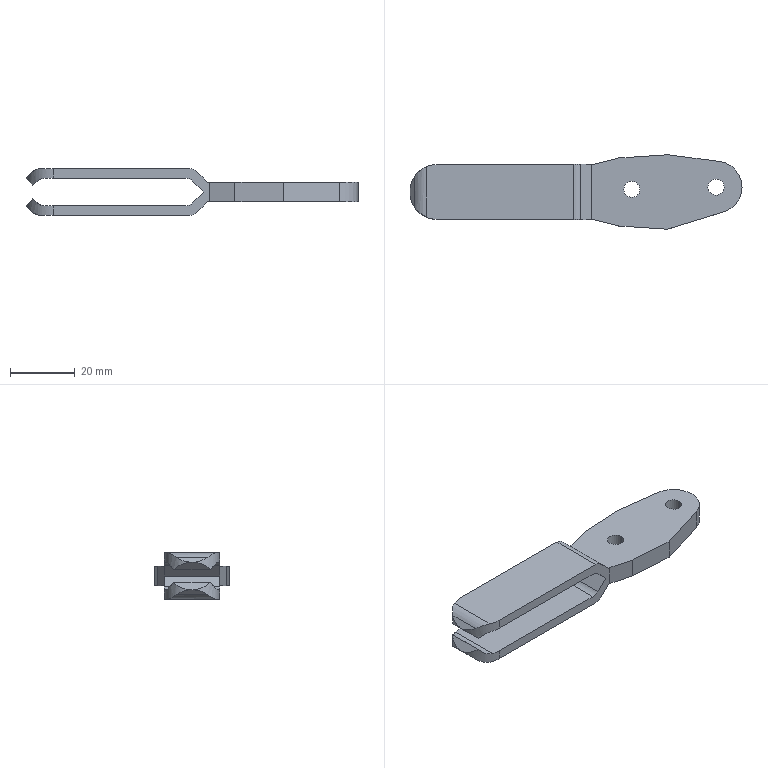Part | STEP file | Sceond_200_APVM-6 | 1 solid | 42 faces | box 102.5 x 23 x 14.5 mm | volume 10818 mm3 | plane 24 | cylinder 18 | commonest cylinder face diameters 5 x4 6 x4 17 x4 8 x2 10 x2 16 x2